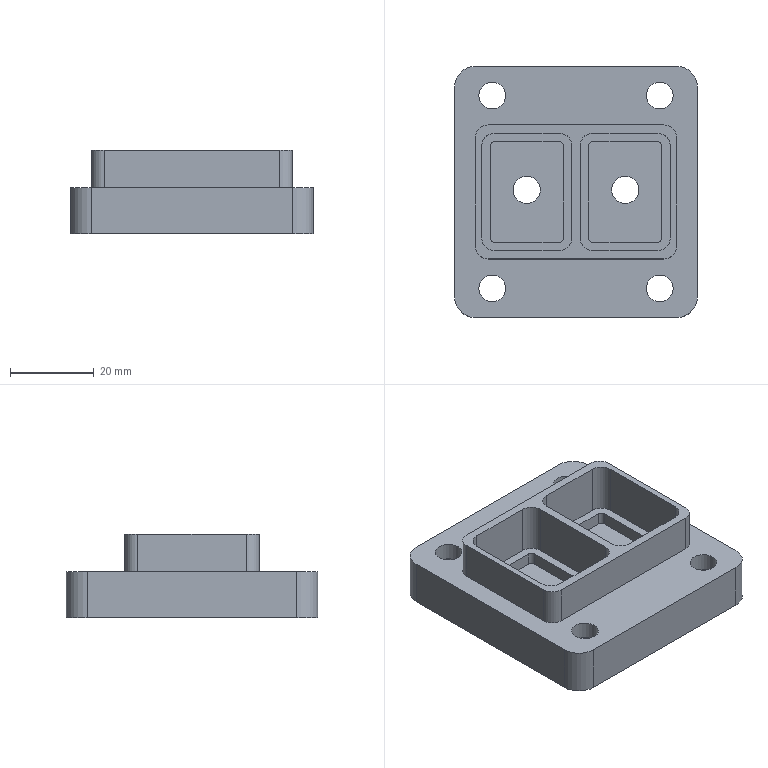Part | NX | features BREP 1 | 1 solid | 69 faces | box 58 x 60 x 20 mm | volume 31793 mm3 | plane 35 | cylinder 34 | commonest cylinder face diameters 6 x12 2 x8 6.4 x4 10 x4 10.5 x4 6.5 x2